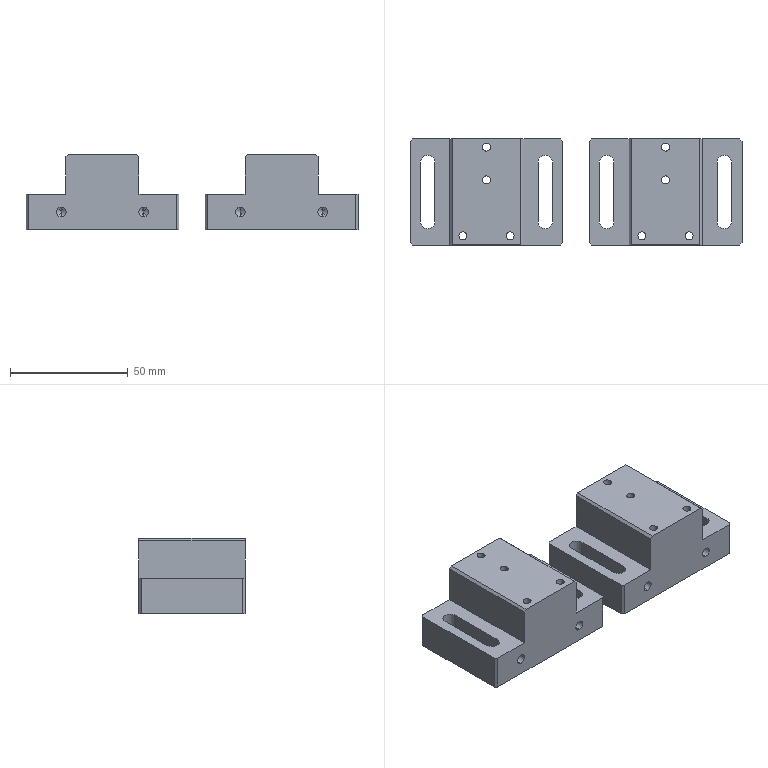NC program | NX | posted with a generic post | part box 140.92 x 45 x 32 mm
Lines 19 to 865 of 6583:
(ZLEVEL_PROFILE , TOOL : D10)
N36 T15 M6
N38 G54
N40 G17 G0 G90 X146.02 Y7.771 S9500 M3
N42 G43 Z30. H15
N44 Z1.5
N46 G94 G1 Y0.406 Z1.114 F1000.
N48 X145.66 Y-1.003 Z1.038
N50 X144.918 Y-2.255 Z0.962
N52 X143.175 Y-3.998 Z0.832
N54 X141.923 Y-4.74 Z0.756
N56 X140.514 Y-5.1 Z0.68
N58 X108.46 Z-1.
N60 X76.96 F3000.
N62 G2 X73.354 Y-3.606 R5.1
N64 G1 X72.394 Y-2.646
N66 G2 X70.9 Y0.96 R5.1
N68 G1 Y44.04
N70 G2 X72.394 Y47.646 R5.1
N72 G1 X73.354 Y48.606
N74 G2 X76.96 Y50.1 R5.1
N76 G1 X139.96
N78 G2 X143.566 Y48.606 R5.1
N80 G1 X144.526 Y47.646
N82 G2 X146.02 Y44.04 R5.1
N84 G1 Y0.96
N86 G2 X144.526 Y-2.646 R5.1
N88 G1 X143.566 Y-3.606
N90 G2 X139.96 Y-5.1 R5.1
N92 G1 X108.46
N94 X76.96 Z-1.126
N96 X76.46 Y-5.075 Z-1.128
N98 X75.965 Y-5.002 Z-1.13
N100 X75.48 Y-4.88 Z-1.132
N102 X75.008 Y-4.712 Z-1.134
N104 X74.556 Y-4.498 Z-1.136
N106 X74.127 Y-4.24 Z-1.138
N108 X73.725 Y-3.942 Z-1.14
N110 X73.354 Y-3.606 Z-1.142
N112 X72.394 Y-2.646 Z-1.148
N114 X72.058 Y-2.275 Z-1.15
N116 X71.76 Y-1.873 Z-1.152
N118 X71.502 Y-1.444 Z-1.154
N120 X71.288 Y-0.992 Z-1.156
N122 X71.12 Y-0.52 Z-1.158
N124 X70.998 Y-0.035 Z-1.16
N126 X70.925 Y0.46 Z-1.162
N128 X70.9 Y0.96 Z-1.164
N130 Y44.04 Z-1.336
N132 X70.925 Y44.54 Z-1.338
N134 X70.998 Y45.035 Z-1.34
N136 X71.12 Y45.52 Z-1.342
N138 X71.288 Y45.992 Z-1.344
N140 X71.502 Y46.444 Z-1.346
N142 X71.76 Y46.873 Z-1.348
N144 X72.058 Y47.275 Z-1.35
N146 X72.394 Y47.646 Z-1.352
N148 X73.354 Y48.606 Z-1.358
N150 X73.725 Y48.942 Z-1.36
N152 X74.127 Y49.24 Z-1.362
N154 X74.556 Y49.498 Z-1.364
N156 X75.008 Y49.712 Z-1.366
N158 X75.48 Y49.88 Z-1.368
N160 X75.965 Y50.002 Z-1.37
N162 X76.46 Y50.075 Z-1.372
N164 X76.96 Y50.1 Z-1.374
N166 X139.96 Z-1.626
N168 X140.46 Y50.075 Z-1.628
N170 X140.955 Y50.002 Z-1.63
N172 X141.44 Y49.88 Z-1.632
N174 X141.912 Y49.712 Z-1.634
N176 X142.364 Y49.498 Z-1.636
N178 X142.793 Y49.24 Z-1.638
N180 X143.195 Y48.942 Z-1.64
N182 X143.566 Y48.606 Z-1.642
N184 X144.526 Y47.646 Z-1.648
N186 X144.862 Y47.275 Z-1.65
N188 X145.16 Y46.873 Z-1.652
N190 X145.418 Y46.444 Z-1.654
N192 X145.632 Y45.992 Z-1.656
N194 X145.8 Y45.52 Z-1.658
N196 X145.922 Y45.035 Z-1.66
N198 X145.995 Y44.54 Z-1.662
N200 X146.02 Y44.04 Z-1.664
N202 Y0.96 Z-1.836
N204 X145.995 Y0.46 Z-1.838
N206 X145.922 Y-0.035 Z-1.84
N208 X145.8 Y-0.52 Z-1.842
N210 X145.632 Y-0.992 Z-1.844
N212 X145.418 Y-1.444 Z-1.846
N214 X145.16 Y-1.873 Z-1.848
N216 X144.862 Y-2.275 Z-1.85
N218 X144.526 Y-2.646 Z-1.852
N220 X143.566 Y-3.606 Z-1.858
N222 X143.195 Y-3.942 Z-1.86
N224 X142.793 Y-4.24 Z-1.862
N226 X142.364 Y-4.498 Z-1.864
N228 X141.912 Y-4.712 Z-1.866
N230 X141.44 Y-4.88 Z-1.868
N232 X140.955 Y-5.002 Z-1.87
N234 X140.46 Y-5.075 Z-1.872
N236 X139.96 Y-5.1 Z-1.874
N238 X108.46 Z-2.
N240 X76.96 Z-2.126
N242 X76.46 Y-5.075 Z-2.128
N244 X75.965 Y-5.002 Z-2.13
N246 X75.48 Y-4.88 Z-2.132
N248 X75.008 Y-4.712 Z-2.134
N250 X74.556 Y-4.498 Z-2.136
N252 X74.127 Y-4.24 Z-2.138
N254 X73.725 Y-3.942 Z-2.14
N256 X73.354 Y-3.606 Z-2.142
N258 X72.394 Y-2.646 Z-2.148
N260 X72.058 Y-2.275 Z-2.15
N262 X71.76 Y-1.873 Z-2.152
N264 X71.502 Y-1.444 Z-2.154
N266 X71.288 Y-0.992 Z-2.156
N268 X71.12 Y-0.52 Z-2.158
N270 X70.998 Y-0.035 Z-2.16
N272 X70.925 Y0.46 Z-2.162
N274 X70.9 Y0.96 Z-2.164
N276 Y44.04 Z-2.336
N278 X70.925 Y44.54 Z-2.338
N280 X70.998 Y45.035 Z-2.34
N282 X71.12 Y45.52 Z-2.342
N284 X71.288 Y45.992 Z-2.344
N286 X71.502 Y46.444 Z-2.346
N288 X71.76 Y46.873 Z-2.348
N290 X72.058 Y47.275 Z-2.35
N292 X72.394 Y47.646 Z-2.352
N294 X73.354 Y48.606 Z-2.358
N296 X73.725 Y48.942 Z-2.36
N298 X74.127 Y49.24 Z-2.362
N300 X74.556 Y49.498 Z-2.364
N302 X75.008 Y49.712 Z-2.366
N304 X75.48 Y49.88 Z-2.368
N306 X75.965 Y50.002 Z-2.37
N308 X76.46 Y50.075 Z-2.372
N310 X76.96 Y50.1 Z-2.374
N312 X139.96 Z-2.626
N314 X140.46 Y50.075 Z-2.628
N316 X140.955 Y50.002 Z-2.63
N318 X141.44 Y49.88 Z-2.632
N320 X141.912 Y49.712 Z-2.634
N322 X142.364 Y49.498 Z-2.636
N324 X142.793 Y49.24 Z-2.638
N326 X143.195 Y48.942 Z-2.64
N328 X143.566 Y48.606 Z-2.642
N330 X144.526 Y47.646 Z-2.648
N332 X144.862 Y47.275 Z-2.65
N334 X145.16 Y46.873 Z-2.652
N336 X145.418 Y46.444 Z-2.654
N338 X145.632 Y45.992 Z-2.656
N340 X145.8 Y45.52 Z-2.658
N342 X145.922 Y45.035 Z-2.66
N344 X145.995 Y44.54 Z-2.662
N346 X146.02 Y44.04 Z-2.664
N348 Y0.96 Z-2.836
N350 X145.995 Y0.46 Z-2.838
N352 X145.922 Y-0.035 Z-2.84
N354 X145.8 Y-0.52 Z-2.842
N356 X145.632 Y-0.992 Z-2.844
N358 X145.418 Y-1.444 Z-2.846
N360 X145.16 Y-1.873 Z-2.848
N362 X144.862 Y-2.275 Z-2.85
N364 X144.526 Y-2.646 Z-2.852
N366 X143.566 Y-3.606 Z-2.858
N368 X143.195 Y-3.942 Z-2.86
N370 X142.793 Y-4.24 Z-2.862
N372 X142.364 Y-4.498 Z-2.864
N374 X141.912 Y-4.712 Z-2.866
N376 X141.44 Y-4.88 Z-2.868
N378 X140.955 Y-5.002 Z-2.87
N380 X140.46 Y-5.075 Z-2.872
N382 X139.96 Y-5.1 Z-2.874
N384 X108.46 Z-3.
N386 X76.96 Z-3.126
N388 X76.46 Y-5.075 Z-3.128
N390 X75.965 Y-5.002 Z-3.13
N392 X75.48 Y-4.88 Z-3.132
N394 X75.008 Y-4.712 Z-3.134
N396 X74.556 Y-4.498 Z-3.136
N398 X74.127 Y-4.24 Z-3.138
N400 X73.725 Y-3.942 Z-3.14
N402 X73.354 Y-3.606 Z-3.142
N404 X72.394 Y-2.646 Z-3.148
N406 X72.058 Y-2.275 Z-3.15
N408 X71.76 Y-1.873 Z-3.152
N410 X71.502 Y-1.444 Z-3.154
N412 X71.288 Y-0.992 Z-3.156
N414 X71.12 Y-0.52 Z-3.158
N416 X70.998 Y-0.035 Z-3.16
N418 X70.925 Y0.46 Z-3.162
N420 X70.9 Y0.96 Z-3.164
N422 Y44.04 Z-3.336
N424 X70.925 Y44.54 Z-3.338
N426 X70.998 Y45.035 Z-3.34
N428 X71.12 Y45.52 Z-3.342
N430 X71.288 Y45.992 Z-3.344
N432 X71.502 Y46.444 Z-3.346
N434 X71.76 Y46.873 Z-3.348
N436 X72.058 Y47.275 Z-3.35
N438 X72.394 Y47.646 Z-3.352
N440 X73.354 Y48.606 Z-3.358
N442 X73.725 Y48.942 Z-3.36
N444 X74.127 Y49.24 Z-3.362
N446 X74.556 Y49.498 Z-3.364
N448 X75.008 Y49.712 Z-3.366
N450 X75.48 Y49.88 Z-3.368
N452 X75.965 Y50.002 Z-3.37
N454 X76.46 Y50.075 Z-3.372
N456 X76.96 Y50.1 Z-3.374
N458 X139.96 Z-3.626
N460 X140.46 Y50.075 Z-3.628
N462 X140.955 Y50.002 Z-3.63
N464 X141.44 Y49.88 Z-3.632
N466 X141.912 Y49.712 Z-3.634
N468 X142.364 Y49.498 Z-3.636
N470 X142.793 Y49.24 Z-3.638
N472 X143.195 Y48.942 Z-3.64
N474 X143.566 Y48.606 Z-3.642
N476 X144.526 Y47.646 Z-3.648
N478 X144.862 Y47.275 Z-3.65
N480 X145.16 Y46.873 Z-3.652
N482 X145.418 Y46.444 Z-3.654
N484 X145.632 Y45.992 Z-3.656
N486 X145.8 Y45.52 Z-3.658
N488 X145.922 Y45.035 Z-3.66
N490 X145.995 Y44.54 Z-3.662
N492 X146.02 Y44.04 Z-3.664
N494 Y0.96 Z-3.836
N496 X145.995 Y0.46 Z-3.838
N498 X145.922 Y-0.035 Z-3.84
N500 X145.8 Y-0.52 Z-3.842
N502 X145.632 Y-0.992 Z-3.844
N504 X145.418 Y-1.444 Z-3.846
N506 X145.16 Y-1.873 Z-3.848
N508 X144.862 Y-2.275 Z-3.85
N510 X144.526 Y-2.646 Z-3.852
N512 X143.566 Y-3.606 Z-3.858
N514 X143.195 Y-3.942 Z-3.86
N516 X142.793 Y-4.24 Z-3.862
N518 X142.364 Y-4.498 Z-3.864
N520 X141.912 Y-4.712 Z-3.866
N522 X141.44 Y-4.88 Z-3.868
N524 X140.955 Y-5.002 Z-3.87
N526 X140.46 Y-5.075 Z-3.872
N528 X139.96 Y-5.1 Z-3.874
N530 X108.46 Z-4.
N532 X76.96 Z-4.126
N534 X76.46 Y-5.075 Z-4.128
N536 X75.965 Y-5.002 Z-4.13
N538 X75.48 Y-4.88 Z-4.132
N540 X75.008 Y-4.712 Z-4.134
N542 X74.556 Y-4.498 Z-4.136
N544 X74.127 Y-4.24 Z-4.138
N546 X73.725 Y-3.942 Z-4.14
N548 X73.354 Y-3.606 Z-4.142
N550 X72.394 Y-2.646 Z-4.148
N552 X72.058 Y-2.275 Z-4.15
N554 X71.76 Y-1.873 Z-4.152
N556 X71.502 Y-1.444 Z-4.154
N558 X71.288 Y-0.992 Z-4.156
N560 X71.12 Y-0.52 Z-4.158
N562 X70.998 Y-0.035 Z-4.16
N564 X70.925 Y0.46 Z-4.162
N566 X70.9 Y0.96 Z-4.164
N568 Y44.04 Z-4.336
N570 X70.925 Y44.54 Z-4.338
N572 X70.998 Y45.035 Z-4.34
N574 X71.12 Y45.52 Z-4.342
N576 X71.288 Y45.992 Z-4.344
N578 X71.502 Y46.444 Z-4.346
N580 X71.76 Y46.873 Z-4.348
N582 X72.058 Y47.275 Z-4.35
N584 X72.394 Y47.646 Z-4.352
N586 X73.354 Y48.606 Z-4.358
N588 X73.725 Y48.942 Z-4.36
N590 X74.127 Y49.24 Z-4.362
N592 X74.556 Y49.498 Z-4.364
N594 X75.008 Y49.712 Z-4.366
N596 X75.48 Y49.88 Z-4.368
N598 X75.965 Y50.002 Z-4.37
N600 X76.46 Y50.075 Z-4.372
N602 X76.96 Y50.1 Z-4.374
N604 X139.96 Z-4.626
N606 X140.46 Y50.075 Z-4.628
N608 X140.955 Y50.002 Z-4.63
N610 X141.44 Y49.88 Z-4.632
N612 X141.912 Y49.712 Z-4.634
N614 X142.364 Y49.498 Z-4.636
N616 X142.793 Y49.24 Z-4.638
N618 X143.195 Y48.942 Z-4.64
N620 X143.566 Y48.606 Z-4.642
N622 X144.526 Y47.646 Z-4.648
N624 X144.862 Y47.275 Z-4.65
N626 X145.16 Y46.873 Z-4.652
N628 X145.418 Y46.444 Z-4.654
N630 X145.632 Y45.992 Z-4.656
N632 X145.8 Y45.52 Z-4.658
N634 X145.922 Y45.035 Z-4.66
N636 X145.995 Y44.54 Z-4.662
N638 X146.02 Y44.04 Z-4.664
N640 Y0.96 Z-4.836
N642 X145.995 Y0.46 Z-4.838
N644 X145.922 Y-0.035 Z-4.84
N646 X145.8 Y-0.52 Z-4.842
N648 X145.632 Y-0.992 Z-4.844
N650 X145.418 Y-1.444 Z-4.846
N652 X145.16 Y-1.873 Z-4.848
N654 X144.862 Y-2.275 Z-4.85
N656 X144.526 Y-2.646 Z-4.852
N658 X143.566 Y-3.606 Z-4.858
N660 X143.195 Y-3.942 Z-4.86
N662 X142.793 Y-4.24 Z-4.862
N664 X142.364 Y-4.498 Z-4.864
N666 X141.912 Y-4.712 Z-4.866
N668 X141.44 Y-4.88 Z-4.868
N670 X140.955 Y-5.002 Z-4.87
N672 X140.46 Y-5.075 Z-4.872
N674 X139.96 Y-5.1 Z-4.874
N676 X108.46 Z-5.
N678 X76.96 Z-5.126
N680 X76.46 Y-5.075 Z-5.128
N682 X75.965 Y-5.002 Z-5.13
N684 X75.48 Y-4.88 Z-5.132
N686 X75.008 Y-4.712 Z-5.134
N688 X74.556 Y-4.498 Z-5.136
N690 X74.127 Y-4.24 Z-5.138
N692 X73.725 Y-3.942 Z-5.14
N694 X73.354 Y-3.606 Z-5.142
N696 X72.394 Y-2.646 Z-5.148
N698 X72.058 Y-2.275 Z-5.15
N700 X71.76 Y-1.873 Z-5.152
N702 X71.502 Y-1.444 Z-5.154
N704 X71.288 Y-0.992 Z-5.156
N706 X71.12 Y-0.52 Z-5.158
N708 X70.998 Y-0.035 Z-5.16
N710 X70.925 Y0.46 Z-5.162
N712 X70.9 Y0.96 Z-5.164
N714 Y44.04 Z-5.336
N716 X70.925 Y44.54 Z-5.338
N718 X70.998 Y45.035 Z-5.34
N720 X71.12 Y45.52 Z-5.342
N722 X71.288 Y45.992 Z-5.344
N724 X71.502 Y46.444 Z-5.346
N726 X71.76 Y46.873 Z-5.348
N728 X72.058 Y47.275 Z-5.35
N730 X72.394 Y47.646 Z-5.352
N732 X73.354 Y48.606 Z-5.358
N734 X73.725 Y48.942 Z-5.36
N736 X74.127 Y49.24 Z-5.362
N738 X74.556 Y49.498 Z-5.364
N740 X75.008 Y49.712 Z-5.366
N742 X75.48 Y49.88 Z-5.368
N744 X75.965 Y50.002 Z-5.37
N746 X76.46 Y50.075 Z-5.372
N748 X76.96 Y50.1 Z-5.374
N750 X139.96 Z-5.626
N752 X140.46 Y50.075 Z-5.628
N754 X140.955 Y50.002 Z-5.63
N756 X141.44 Y49.88 Z-5.632
N758 X141.912 Y49.712 Z-5.634
N760 X142.364 Y49.498 Z-5.636
N762 X142.793 Y49.24 Z-5.638
N764 X143.195 Y48.942 Z-5.64
N766 X143.566 Y48.606 Z-5.642
N768 X144.526 Y47.646 Z-5.648
N770 X144.862 Y47.275 Z-5.65
N772 X145.16 Y46.873 Z-5.652
N774 X145.418 Y46.444 Z-5.654
N776 X145.632 Y45.992 Z-5.656
N778 X145.8 Y45.52 Z-5.658
N780 X145.922 Y45.035 Z-5.66
N782 X145.995 Y44.54 Z-5.662
N784 X146.02 Y44.04 Z-5.664
N786 Y0.96 Z-5.836
N788 X145.995 Y0.46 Z-5.838
N790 X145.922 Y-0.035 Z-5.84
N792 X145.8 Y-0.52 Z-5.842
N794 X145.632 Y-0.992 Z-5.844
N796 X145.418 Y-1.444 Z-5.846
N798 X145.16 Y-1.873 Z-5.848
N800 X144.862 Y-2.275 Z-5.85
N802 X144.526 Y-2.646 Z-5.852
N804 X143.566 Y-3.606 Z-5.858
N806 X143.195 Y-3.942 Z-5.86
N808 X142.793 Y-4.24 Z-5.862
N810 X142.364 Y-4.498 Z-5.864
N812 X141.912 Y-4.712 Z-5.866
N814 X141.44 Y-4.88 Z-5.868
N816 X140.955 Y-5.002 Z-5.87
N818 X140.46 Y-5.075 Z-5.872
N820 X139.96 Y-5.1 Z-5.874
N822 X108.46 Z-6.
N824 X76.96 Z-6.126
N826 X76.46 Y-5.075 Z-6.128
N828 X75.965 Y-5.002 Z-6.13
N830 X75.48 Y-4.88 Z-6.132
N832 X75.008 Y-4.712 Z-6.134
N834 X74.556 Y-4.498 Z-6.136
N836 X74.127 Y-4.24 Z-6.138
N838 X73.725 Y-3.942 Z-6.14
N840 X73.354 Y-3.606 Z-6.142
N842 X72.394 Y-2.646 Z-6.148
N844 X72.058 Y-2.275 Z-6.15
N846 X71.76 Y-1.873 Z-6.152
N848 X71.502 Y-1.444 Z-6.154
N850 X71.288 Y-0.992 Z-6.156
N852 X71.12 Y-0.52 Z-6.158
N854 X70.998 Y-0.035 Z-6.16
N856 X70.925 Y0.46 Z-6.162
N858 X70.9 Y0.96 Z-6.164
N860 Y44.04 Z-6.336
N862 X70.925 Y44.54 Z-6.338
N864 X70.998 Y45.035 Z-6.34
N866 X71.12 Y45.52 Z-6.342
N868 X71.288 Y45.992 Z-6.344
N870 X71.502 Y46.444 Z-6.346
N872 X71.76 Y46.873 Z-6.348
N874 X72.058 Y47.275 Z-6.35
N876 X72.394 Y47.646 Z-6.352
N878 X73.354 Y48.606 Z-6.358
N880 X73.725 Y48.942 Z-6.36
N882 X74.127 Y49.24 Z-6.362
N884 X74.556 Y49.498 Z-6.364
N886 X75.008 Y49.712 Z-6.366
N888 X75.48 Y49.88 Z-6.368
N890 X75.965 Y50.002 Z-6.37
N892 X76.46 Y50.075 Z-6.372
N894 X76.96 Y50.1 Z-6.374
N896 X139.96 Z-6.626
N898 X140.46 Y50.075 Z-6.628
N900 X140.955 Y50.002 Z-6.63
N902 X141.44 Y49.88 Z-6.632
N904 X141.912 Y49.712 Z-6.634
N906 X142.364 Y49.498 Z-6.636
N908 X142.793 Y49.24 Z-6.638
N910 X143.195 Y48.942 Z-6.64
N912 X143.566 Y48.606 Z-6.642
N914 X144.526 Y47.646 Z-6.648
N916 X144.862 Y47.275 Z-6.65
N918 X145.16 Y46.873 Z-6.652
N920 X145.418 Y46.444 Z-6.654
N922 X145.632 Y45.992 Z-6.656
N924 X145.8 Y45.52 Z-6.658
N926 X145.922 Y45.035 Z-6.66
N928 X145.995 Y44.54 Z-6.662
N930 X146.02 Y44.04 Z-6.664
N932 Y0.96 Z-6.836
N934 X145.995 Y0.46 Z-6.838
N936 X145.922 Y-0.035 Z-6.84
N938 X145.8 Y-0.52 Z-6.842
N940 X145.632 Y-0.992 Z-6.844
N942 X145.418 Y-1.444 Z-6.846
N944 X145.16 Y-1.873 Z-6.848
N946 X144.862 Y-2.275 Z-6.85
N948 X144.526 Y-2.646 Z-6.852
N950 X143.566 Y-3.606 Z-6.858
N952 X143.195 Y-3.942 Z-6.86
N954 X142.793 Y-4.24 Z-6.862
N956 X142.364 Y-4.498 Z-6.864
N958 X141.912 Y-4.712 Z-6.866
N960 X141.44 Y-4.88 Z-6.868
N962 X140.955 Y-5.002 Z-6.87
N964 X140.46 Y-5.075 Z-6.872
N966 X139.96 Y-5.1 Z-6.874
N968 X108.46 Z-7.
N970 X76.96 Z-7.126
N972 X76.46 Y-5.075 Z-7.128
N974 X75.965 Y-5.002 Z-7.13
N976 X75.48 Y-4.88 Z-7.132
N978 X75.008 Y-4.712 Z-7.134
N980 X74.556 Y-4.498 Z-7.136
N982 X74.127 Y-4.24 Z-7.138
N984 X73.725 Y-3.942 Z-7.14
N986 X73.354 Y-3.606 Z-7.142
N988 X72.394 Y-2.646 Z-7.148
N990 X72.058 Y-2.275 Z-7.15
N992 X71.76 Y-1.873 Z-7.152
N994 X71.502 Y-1.444 Z-7.154
N996 X71.288 Y-0.992 Z-7.156
N998 X71.12 Y-0.52 Z-7.158
N1000 X70.998 Y-0.035 Z-7.16
N1002 X70.925 Y0.46 Z-7.162
N1004 X70.9 Y0.96 Z-7.164
N1006 Y44.04 Z-7.336
N1008 X70.925 Y44.54 Z-7.338
N1010 X70.998 Y45.035 Z-7.34
N1012 X71.12 Y45.52 Z-7.342
N1014 X71.288 Y45.992 Z-7.344
N1016 X71.502 Y46.444 Z-7.346
N1018 X71.76 Y46.873 Z-7.348
N1020 X72.058 Y47.275 Z-7.35
N1022 X72.394 Y47.646 Z-7.352
N1024 X73.354 Y48.606 Z-7.358
N1026 X73.725 Y48.942 Z-7.36
N1028 X74.127 Y49.24 Z-7.362
N1030 X74.556 Y49.498 Z-7.364
N1032 X75.008 Y49.712 Z-7.366
N1034 X75.48 Y49.88 Z-7.368
N1036 X75.965 Y50.002 Z-7.37
N1038 X76.46 Y50.075 Z-7.372
N1040 X76.96 Y50.1 Z-7.374
N1042 X139.96 Z-7.626
N1044 X140.46 Y50.075 Z-7.628
N1046 X140.955 Y50.002 Z-7.63
N1048 X141.44 Y49.88 Z-7.632
N1050 X141.912 Y49.712 Z-7.634
N1052 X142.364 Y49.498 Z-7.636
N1054 X142.793 Y49.24 Z-7.638
N1056 X143.195 Y48.942 Z-7.64
N1058 X143.566 Y48.606 Z-7.642
N1060 X144.526 Y47.646 Z-7.648
N1062 X144.862 Y47.275 Z-7.65
N1064 X145.16 Y46.873 Z-7.652
N1066 X145.418 Y46.444 Z-7.654
N1068 X145.632 Y45.992 Z-7.656
N1070 X145.8 Y45.52 Z-7.658
N1072 X145.922 Y45.035 Z-7.66
N1074 X145.995 Y44.54 Z-7.662
N1076 X146.02 Y44.04 Z-7.664
N1078 Y0.96 Z-7.836
N1080 X145.995 Y0.46 Z-7.838
N1082 X145.922 Y-0.035 Z-7.84
N1084 X145.8 Y-0.52 Z-7.842
N1086 X145.632 Y-0.992 Z-7.844
N1088 X145.418 Y-1.444 Z-7.846
N1090 X145.16 Y-1.873 Z-7.848
N1092 X144.862 Y-2.275 Z-7.85
N1094 X144.526 Y-2.646 Z-7.852
N1096 X143.566 Y-3.606 Z-7.858
N1098 X143.195 Y-3.942 Z-7.86
N1100 X142.793 Y-4.24 Z-7.862
N1102 X142.364 Y-4.498 Z-7.864
N1104 X141.912 Y-4.712 Z-7.866
N1106 X141.44 Y-4.88 Z-7.868
N1108 X140.955 Y-5.002 Z-7.87
N1110 X140.46 Y-5.075 Z-7.872
N1112 X139.96 Y-5.1 Z-7.874
N1114 X108.46 Z-8.
N1116 X76.96 Z-8.126
N1118 X76.46 Y-5.075 Z-8.128
N1120 X75.965 Y-5.002 Z-8.13
N1122 X75.48 Y-4.88 Z-8.132
N1124 X75.008 Y-4.712 Z-8.134
N1126 X74.556 Y-4.498 Z-8.136
N1128 X74.127 Y-4.24 Z-8.138
N1130 X73.725 Y-3.942 Z-8.14
N1132 X73.354 Y-3.606 Z-8.142
N1134 X72.394 Y-2.646 Z-8.148
N1136 X72.058 Y-2.275 Z-8.15
N1138 X71.76 Y-1.873 Z-8.152
N1140 X71.502 Y-1.444 Z-8.154
N1142 X71.288 Y-0.992 Z-8.156
N1144 X71.12 Y-0.52 Z-8.158
N1146 X70.998 Y-0.035 Z-8.16
N1148 X70.925 Y0.46 Z-8.162
N1150 X70.9 Y0.96 Z-8.164
N1152 Y44.04 Z-8.336
N1154 X70.925 Y44.54 Z-8.338
N1156 X70.998 Y45.035 Z-8.34
N1158 X71.12 Y45.52 Z-8.342
N1160 X71.288 Y45.992 Z-8.344
N1162 X71.502 Y46.444 Z-8.346
N1164 X71.76 Y46.873 Z-8.348
N1166 X72.058 Y47.275 Z-8.35
N1168 X72.394 Y47.646 Z-8.352
N1170 X73.354 Y48.606 Z-8.358
N1172 X73.725 Y48.942 Z-8.36
N1174 X74.127 Y49.24 Z-8.362
N1176 X74.556 Y49.498 Z-8.364
N1178 X75.008 Y49.712 Z-8.366
N1180 X75.48 Y49.88 Z-8.368
N1182 X75.965 Y50.002 Z-8.37
N1184 X76.46 Y50.075 Z-8.372
N1186 X76.96 Y50.1 Z-8.374
N1188 X139.96 Z-8.626
N1190 X140.46 Y50.075 Z-8.628
N1192 X140.955 Y50.002 Z-8.63
N1194 X141.44 Y49.88 Z-8.632
N1196 X141.912 Y49.712 Z-8.634
N1198 X142.364 Y49.498 Z-8.636
N1200 X142.793 Y49.24 Z-8.638
N1202 X143.195 Y48.942 Z-8.64
N1204 X143.566 Y48.606 Z-8.642
N1206 X144.526 Y47.646 Z-8.648
N1208 X144.862 Y47.275 Z-8.65
N1210 X145.16 Y46.873 Z-8.652
N1212 X145.418 Y46.444 Z-8.654
N1214 X145.632 Y45.992 Z-8.656
N1216 X145.8 Y45.52 Z-8.658
N1218 X145.922 Y45.035 Z-8.66
N1220 X145.995 Y44.54 Z-8.662
N1222 X146.02 Y44.04 Z-8.664
N1224 Y0.96 Z-8.836
N1226 X145.995 Y0.46 Z-8.838
N1228 X145.922 Y-0.035 Z-8.84
N1230 X145.8 Y-0.52 Z-8.842
N1232 X145.632 Y-0.992 Z-8.844
N1234 X145.418 Y-1.444 Z-8.846
N1236 X145.16 Y-1.873 Z-8.848
N1238 X144.862 Y-2.275 Z-8.85
N1240 X144.526 Y-2.646 Z-8.852
N1242 X143.566 Y-3.606 Z-8.858
N1244 X143.195 Y-3.942 Z-8.86
N1246 X142.793 Y-4.24 Z-8.862
N1248 X142.364 Y-4.498 Z-8.864
N1250 X141.912 Y-4.712 Z-8.866
N1252 X141.44 Y-4.88 Z-8.868
N1254 X140.955 Y-5.002 Z-8.87
N1256 X140.46 Y-5.075 Z-8.872
N1258 X139.96 Y-5.1 Z-8.874
N1260 X108.46 Z-9.
N1262 X76.96 Z-9.126
N1264 X76.46 Y-5.075 Z-9.128
N1266 X75.965 Y-5.002 Z-9.13
N1268 X75.48 Y-4.88 Z-9.132
N1270 X75.008 Y-4.712 Z-9.134
N1272 X74.556 Y-4.498 Z-9.136
N1274 X74.127 Y-4.24 Z-9.138
N1276 X73.725 Y-3.942 Z-9.14
N1278 X73.354 Y-3.606 Z-9.142
N1280 X72.394 Y-2.646 Z-9.148
N1282 X72.058 Y-2.275 Z-9.15
N1284 X71.76 Y-1.873 Z-9.152
N1286 X71.502 Y-1.444 Z-9.154
N1288 X71.288 Y-0.992 Z-9.156
N1290 X71.12 Y-0.52 Z-9.158
N1292 X70.998 Y-0.035 Z-9.16
N1294 X70.925 Y0.46 Z-9.162
N1296 X70.9 Y0.96 Z-9.164
N1298 Y44.04 Z-9.336
N1300 X70.925 Y44.54 Z-9.338
N1302 X70.998 Y45.035 Z-9.34
N1304 X71.12 Y45.52 Z-9.342
N1306 X71.288 Y45.992 Z-9.344
N1308 X71.502 Y46.444 Z-9.346
N1310 X71.76 Y46.873 Z-9.348
N1312 X72.058 Y47.275 Z-9.35
N1314 X72.394 Y47.646 Z-9.352
N1316 X73.354 Y48.606 Z-9.358
N1318 X73.725 Y48.942 Z-9.36
N1320 X74.127 Y49.24 Z-9.362
N1322 X74.556 Y49.498 Z-9.364
N1324 X75.008 Y49.712 Z-9.366
N1326 X75.48 Y49.88 Z-9.368
N1328 X75.965 Y50.002 Z-9.37
N1330 X76.46 Y50.075 Z-9.372
N1332 X76.96 Y50.1 Z-9.374
N1334 X139.96 Z-9.626
N1336 X140.46 Y50.075 Z-9.628
N1338 X140.955 Y50.002 Z-9.63
N1340 X141.44 Y49.88 Z-9.632
N1342 X141.912 Y49.712 Z-9.634
N1344 X142.364 Y49.498 Z-9.636
N1346 X142.793 Y49.24 Z-9.638
N1348 X143.195 Y48.942 Z-9.64
N1350 X143.566 Y48.606 Z-9.642
N1352 X144.526 Y47.646 Z-9.648
N1354 X144.862 Y47.275 Z-9.65
N1356 X145.16 Y46.873 Z-9.652
N1358 X145.418 Y46.444 Z-9.654
N1360 X145.632 Y45.992 Z-9.656
N1362 X145.8 Y45.52 Z-9.658
N1364 X145.922 Y45.035 Z-9.66
N1366 X145.995 Y44.54 Z-9.662
N1368 X146.02 Y44.04 Z-9.664
N1370 Y0.96 Z-9.836
N1372 X145.995 Y0.46 Z-9.838
N1374 X145.922 Y-0.035 Z-9.84
N1376 X145.8 Y-0.52 Z-9.842
N1378 X145.632 Y-0.992 Z-9.844
N1380 X145.418 Y-1.444 Z-9.846
N1382 X145.16 Y-1.873 Z-9.848
N1384 X144.862 Y-2.275 Z-9.85
N1386 X144.526 Y-2.646 Z-9.852
N1388 X143.566 Y-3.606 Z-9.858
N1390 X143.195 Y-3.942 Z-9.86
N1392 X142.793 Y-4.24 Z-9.862
N1394 X142.364 Y-4.498 Z-9.864
N1396 X141.912 Y-4.712 Z-9.866
N1398 X141.44 Y-4.88 Z-9.868
N1400 X140.955 Y-5.002 Z-9.87
N1402 X140.46 Y-5.075 Z-9.872
N1404 X139.96 Y-5.1 Z-9.874
N1406 X108.46 Z-10.
N1408 X76.96 Z-10.126
N1410 X76.46 Y-5.075 Z-10.128
N1412 X75.965 Y-5.002 Z-10.13
N1414 X75.48 Y-4.88 Z-10.132
N1416 X75.008 Y-4.712 Z-10.134
N1418 X74.556 Y-4.498 Z-10.136
N1420 X74.127 Y-4.24 Z-10.138
N1422 X73.725 Y-3.942 Z-10.14
N1424 X73.354 Y-3.606 Z-10.142
N1426 X72.394 Y-2.646 Z-10.148
N1428 X72.058 Y-2.275 Z-10.15
N1430 X71.76 Y-1.873 Z-10.152
N1432 X71.502 Y-1.444 Z-10.154
N1434 X71.288 Y-0.992 Z-10.156
N1436 X71.12 Y-0.52 Z-10.158
N1438 X70.998 Y-0.035 Z-10.16
N1440 X70.925 Y0.46 Z-10.162
N1442 X70.9 Y0.96 Z-10.164
N1444 Y44.04 Z-10.336
N1446 X70.925 Y44.54 Z-10.338
N1448 X70.998 Y45.035 Z-10.34
N1450 X71.12 Y45.52 Z-10.342
N1452 X71.288 Y45.992 Z-10.344
N1454 X71.502 Y46.444 Z-10.346
N1456 X71.76 Y46.873 Z-10.348
N1458 X72.058 Y47.275 Z-10.35
N1460 X72.394 Y47.646 Z-10.352
N1462 X73.354 Y48.606 Z-10.358
N1464 X73.725 Y48.942 Z-10.36
N1466 X74.127 Y49.24 Z-10.362
N1468 X74.556 Y49.498 Z-10.364
N1470 X75.008 Y49.712 Z-10.366
N1472 X75.48 Y49.88 Z-10.368
N1474 X75.965 Y50.002 Z-10.37
N1476 X76.46 Y50.075 Z-10.372
N1478 X76.96 Y50.1 Z-10.374
N1480 X139.96 Z-10.626
N1482 X140.46 Y50.075 Z-10.628
N1484 X140.955 Y50.002 Z-10.63
N1486 X141.44 Y49.88 Z-10.632
N1488 X141.912 Y49.712 Z-10.634
N1490 X142.364 Y49.498 Z-10.636
N1492 X142.793 Y49.24 Z-10.638
N1494 X143.195 Y48.942 Z-10.64
N1496 X143.566 Y48.606 Z-10.642
N1498 X144.526 Y47.646 Z-10.648
N1500 X144.862 Y47.275 Z-10.65
N1502 X145.16 Y46.873 Z-10.652
N1504 X145.418 Y46.444 Z-10.654
N1506 X145.632 Y45.992 Z-10.656
N1508 X145.8 Y45.52 Z-10.658
N1510 X145.922 Y45.035 Z-10.66
N1512 X145.995 Y44.54 Z-10.662
N1514 X146.02 Y44.04 Z-10.664
N1516 Y0.96 Z-10.836
N1518 X145.995 Y0.46 Z-10.838
N1520 X145.922 Y-0.035 Z-10.84
N1522 X145.8 Y-0.52 Z-10.842
N1524 X145.632 Y-0.992 Z-10.844
N1526 X145.418 Y-1.444 Z-10.846
N1528 X145.16 Y-1.873 Z-10.848
N1530 X144.862 Y-2.275 Z-10.85
N1532 X144.526 Y-2.646 Z-10.852
N1534 X143.566 Y-3.606 Z-10.858
N1536 X143.195 Y-3.942 Z-10.86
N1538 X142.793 Y-4.24 Z-10.862
N1540 X142.364 Y-4.498 Z-10.864
N1542 X141.912 Y-4.712 Z-10.866
N1544 X141.44 Y-4.88 Z-10.868
N1546 X140.955 Y-5.002 Z-10.87
N1548 X140.46 Y-5.075 Z-10.872
N1550 X139.96 Y-5.1 Z-10.874
N1552 X108.46 Z-11.
N1554 X76.96 Z-11.126
N1556 X76.46 Y-5.075 Z-11.128
N1558 X75.965 Y-5.002 Z-11.13
N1560 X75.48 Y-4.88 Z-11.132
N1562 X75.008 Y-4.712 Z-11.134
N1564 X74.556 Y-4.498 Z-11.136
N1566 X74.127 Y-4.24 Z-11.138
N1568 X73.725 Y-3.942 Z-11.14
N1570 X73.354 Y-3.606 Z-11.142
N1572 X72.394 Y-2.646 Z-11.148
N1574 X72.058 Y-2.275 Z-11.15
N1576 X71.76 Y-1.873 Z-11.152
N1578 X71.502 Y-1.444 Z-11.154
N1580 X71.288 Y-0.992 Z-11.156
N1582 X71.12 Y-0.52 Z-11.158
N1584 X70.998 Y-0.035 Z-11.16
N1586 X70.925 Y0.46 Z-11.162
N1588 X70.9 Y0.96 Z-11.164
N1590 Y44.04 Z-11.336
N1592 X70.925 Y44.54 Z-11.338
N1594 X70.998 Y45.035 Z-11.34
N1596 X71.12 Y45.52 Z-11.342
N1598 X71.288 Y45.992 Z-11.344
N1600 X71.502 Y46.444 Z-11.346
N1602 X71.76 Y46.873 Z-11.348
N1604 X72.058 Y47.275 Z-11.35
N1606 X72.394 Y47.646 Z-11.352
N1608 X73.354 Y48.606 Z-11.358
N1610 X73.725 Y48.942 Z-11.36
N1612 X74.127 Y49.24 Z-11.362
N1614 X74.556 Y49.498 Z-11.364
N1616 X75.008 Y49.712 Z-11.366
N1618 X75.48 Y49.88 Z-11.368
N1620 X75.965 Y50.002 Z-11.37
N1622 X76.46 Y50.075 Z-11.372
N1624 X76.96 Y50.1 Z-11.374
N1626 X139.96 Z-11.626
N1628 X140.46 Y50.075 Z-11.628
N1630 X140.955 Y50.002 Z-11.63
N1632 X141.44 Y49.88 Z-11.632
N1634 X141.912 Y49.712 Z-11.634
N1636 X142.364 Y49.498 Z-11.636
N1638 X142.793 Y49.24 Z-11.638
N1640 X143.195 Y48.942 Z-11.64
N1642 X143.566 Y48.606 Z-11.642
N1644 X144.526 Y47.646 Z-11.648
N1646 X144.862 Y47.275 Z-11.65
N1648 X145.16 Y46.873 Z-11.652
N1650 X145.418 Y46.444 Z-11.654
N1652 X145.632 Y45.992 Z-11.656
N1654 X145.8 Y45.52 Z-11.658
N1656 X145.922 Y45.035 Z-11.66
N1658 X145.995 Y44.54 Z-11.662
N1660 X146.02 Y44.04 Z-11.664
N1662 Y0.96 Z-11.836
N1664 X145.995 Y0.46 Z-11.838
N1666 X145.922 Y-0.035 Z-11.84
N1668 X145.8 Y-0.52 Z-11.842
N1670 X145.632 Y-0.992 Z-11.844
N1672 X145.418 Y-1.444 Z-11.846
N1674 X145.16 Y-1.873 Z-11.848
N1676 X144.862 Y-2.275 Z-11.85
N1678 X144.526 Y-2.646 Z-11.852
N1680 X143.566 Y-3.606 Z-11.858
N1682 X143.195 Y-3.942 Z-11.86
N1684 X142.793 Y-4.24 Z-11.862
N1686 X142.364 Y-4.498 Z-11.864
N1688 X141.912 Y-4.712 Z-11.866
N1690 X141.44 Y-4.88 Z-11.868
N1692 X140.955 Y-5.002 Z-11.87
N1694 X140.46 Y-5.075 Z-11.872
N1696 X139.96 Y-5.1 Z-11.874
N1698 X108.46 Z-12.
N1700 X76.96 Z-12.126
N1702 X76.46 Y-5.075 Z-12.128
N1704 X75.965 Y-5.002 Z-12.13
N1706 X75.48 Y-4.88 Z-12.132
N1708 X75.008 Y-4.712 Z-12.134
N1710 X74.556 Y-4.498 Z-12.136
N1712 X74.127 Y-4.24 Z-12.138
N1714 X73.725 Y-3.942 Z-12.14
N1716 X73.354 Y-3.606 Z-12.142
N1718 X72.394 Y-2.646 Z-12.148
N1720 X72.058 Y-2.275 Z-12.15
N1722 X71.76 Y-1.873 Z-12.152